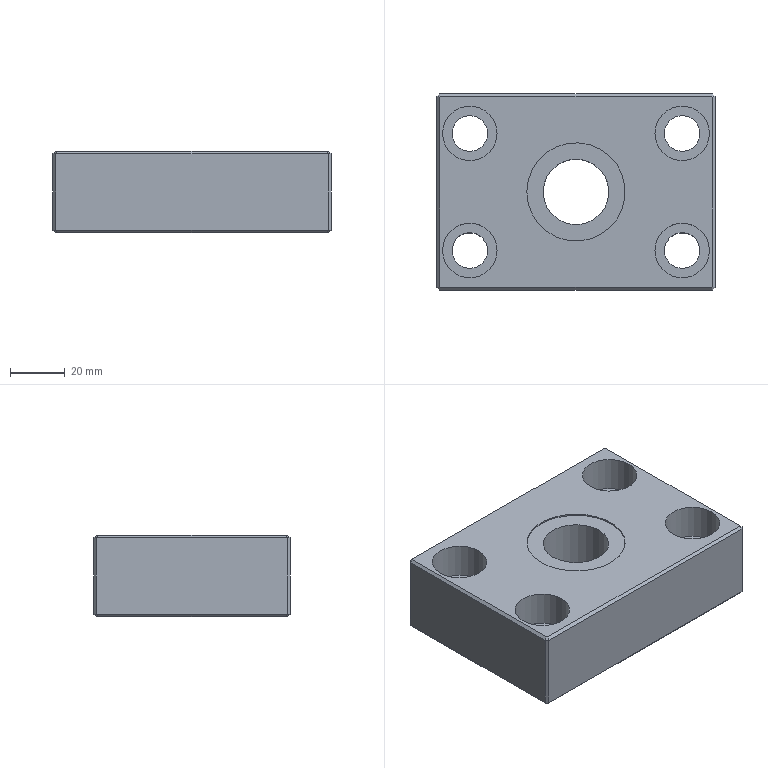NC program | NX | posted with a generic post | part box 102 x 72 x 30 mm
Whole program:
N10 G17 G21 G94 G90
(PLANAR_MILL , TOOL : D80-FACE-MILL)
N12 T01 M6
N14 G53
N16 G17 G0 G90 X96. Y-0.5 S3500 M3
N18 G43 Z20. H1
N20 Z2.03
N22 G94 G1 Z0.03 F800.
N24 X53.
N26 X-53.
N28 X-96.
N30 Z2.03
N32 G0 Z20.
N34 M5
(ADAPTIVE_MILLING , TOOL : D12-36-D12-75-3T-ROUGH)
N36 T02 M6
N38 G53
N40 G17 G0 G90 X-65.022 Y-0.963 S4500 M3
N42 G43 Z20. H2
N44 Z-28.
N46 G94 G1 X-64.873 Y-0.957 Z-28.937 F3000.
N48 X-64.723 Y-0.951 Z-29.308
N50 X-64.573 Y-0.945 Z-29.58
N52 X-64.423 Y-0.939 Z-29.8
N54 X-64.273 Y-0.932 Z-29.984
N56 X-64.123 Y-0.926 Z-30.142
N58 X-63.973 Y-0.92 Z-30.28
N60 X-63.823 Y-0.914 Z-30.4
N62 X-63.673 Y-0.908 Z-30.505
N64 X-63.524 Y-0.902 Z-30.598
N66 X-63.374 Y-0.896 Z-30.679
N68 X-63.224 Y-0.89 Z-30.75
N70 X-63.074 Y-0.884 Z-30.81
N72 X-62.924 Y-0.878 Z-30.862
N74 X-62.774 Y-0.872 Z-30.905
N76 X-62.624 Y-0.866 Z-30.939
N78 X-62.474 Y-0.86 Z-30.966
N80 X-62.325 Y-0.854 Z-30.985
N82 X-62.175 Y-0.848 Z-30.996
N84 X-62.025 Y-0.842 Z-31.
N86 X-60.086 Y-0.763
N88 G3 X-59.024 Y-0.037 R1.213
N90 X-58.336 Y3.017 R10.296
N92 X-58.027 Y11.039 R88.278
N94 G1 X-58.001 Y22.999
N96 G2 X-57.983 Y34.698 R876.175
N98 X-55.786 Y38.926 R6.62
N100 G3 X-54.348 Y40.349 R38.231
N102 G1 X-53.415 Y41.114
N104 X-52.352 Y41.682
N106 X-51.198 Y42.032
N108 G2 X-41.908 Y42.469 R88.797
N110 G1 X-28.858 Y42.499
N112 X49.797
N114 G2 X54.262 Y40.49 R6.403
N116 G3 X55.349 Y39.348 R52.182
N118 G1 X56.114 Y38.415
N120 X56.682 Y37.352
N122 G2 X57.709 Y31.906 R22.458
N124 X57.984 Y22.313 R130.619
N126 G1 X57.999 Y11.513
N128 X57.998 Y-34.397
N130 G2 X56.106 Y-38.609 R6.375
N132 G3 X54.348 Y-40.349 R75.716
N134 G1 X53.415 Y-41.114
N136 X52.352 Y-41.682
N138 X51.198 Y-42.032
N140 G2 X42.058 Y-42.467 R87.641
N142 G1 X28.858 Y-42.499
N144 X-49.901 Y-42.498
N146 G2 X-54.172 Y-40.545 R6.4
N148 G1 X-55.349 Y-39.348
N150 X-56.114 Y-38.415
N152 X-56.682 Y-37.352
N154 G2 X-57.712 Y-31.831 R22.603
N156 X-57.981 Y-22.837 R125.592
N158 G1 X-57.999 Y-11.437
N160 X-57.994 Y30.263
N162 G2 X-57.654 Y31.418 R35.846
N164 X-57.159 Y33.447 R34.168
N166 X-57.031 Y36.201 R19.38
N168 G1 X-56.681 Y37.355
N170 X-56.113 Y38.418
N172 X-55.399 Y39.287
N174 X-56.113 Y38.418
N176 X-56.681 Y37.355
N178 X-57.031 Y36.201
N180 G3 X-57.15 Y33.525 R16.38
N182 G2 X-57.284 Y30.611 R46.933
N184 G3 X-57.399 Y18.162 R360.152
N186 G1 Y-30.651
N188 X-57.15 Y-32.257
N190 Y-35.
N192 X-57.032 Y-36.198
N194 X-57.15 Y-35.
N196 Y35.001
N198 X-57.031 Y36.201
N200 X-56.681 Y37.355
N202 X-56.113 Y38.418
N204 G2 X-53.415 Y41.114 R14.478
N206 G1 X-52.352 Y41.682
N208 X-51.198 Y42.032
N210 X-49.999 Y42.15
N212 X50.001
N214 X51.201 Y42.031
N216 X52.355 Y41.681
N218 X53.418 Y41.113
N220 G2 X56.114 Y38.415 R14.476
N222 G1 X56.682 Y37.352
N224 X57.032 Y36.198
N226 X57.15 Y34.999
N228 Y-35.001
N230 X57.031 Y-36.201
N232 X56.681 Y-37.355
N234 X56.113 Y-38.418
N236 G2 X53.415 Y-41.114 R14.478
N238 G1 X52.352 Y-41.682
N240 X51.198 Y-42.032
N242 X49.999 Y-42.15
N244 X-50.001
N246 X-51.201 Y-42.031
N248 X-52.355 Y-41.681
N250 X-53.418 Y-41.113
N252 G2 X-54.614 Y-40.083 R11.256
N254 G3 X-56.113 Y-39.912 R1.212
N256 G1 X-57.83 Y-40.984
N258 X-57.958 Y-41.063 Z-30.996
N260 X-58.085 Y-41.143 Z-30.985
N262 X-58.212 Y-41.222 Z-30.966
N264 X-58.339 Y-41.302 Z-30.939
N266 X-58.466 Y-41.381 Z-30.905
N268 X-58.594 Y-41.461 Z-30.862
N270 X-58.721 Y-41.54 Z-30.81
N272 X-58.848 Y-41.62 Z-30.75
N274 X-58.975 Y-41.699 Z-30.679
N276 X-59.103 Y-41.779 Z-30.598
N278 X-59.23 Y-41.858 Z-30.505
N280 X-59.357 Y-41.937 Z-30.4
N282 X-59.484 Y-42.017 Z-30.28
N284 X-59.612 Y-42.096 Z-30.142
N286 X-59.739 Y-42.176 Z-29.984
N288 X-59.866 Y-42.255 Z-29.8
N290 X-59.993 Y-42.335 Z-29.58
N292 X-60.12 Y-42.414 Z-29.308
N294 X-60.248 Y-42.494 Z-28.937
N296 X-60.375 Y-42.573 Z-28.
N298 G0 Z20.
N300 X-4.55 Y-2.906
N302 Z3.
N304 G3 X-4.55 Y-2.906 Z2.408 I4.55 J2.908
N306 X-4.55 Y-2.906 Z1.816 I4.55 J2.908
N308 X-4.55 Y-2.906 Z1.223 I4.55 J2.908
N310 X-4.55 Y-2.906 Z0.631 I4.55 J2.908
N312 X-4.55 Y-2.906 Z0.039 I4.55 J2.908
N314 X-4.55 Y-2.906 Z-0.553 I4.55 J2.908
N316 X-4.55 Y-2.906 Z-1.146 I4.55 J2.908
N318 X-4.55 Y-2.906 Z-1.738 I4.55 J2.908
N320 X-4.55 Y-2.906 Z-2.33 I4.55 J2.908
N322 X-4.55 Y-2.906 Z-2.922 I4.55 J2.908
N324 X-4.55 Y-2.906 Z-3.515 I4.55 J2.908
N326 X-4.55 Y-2.906 Z-4.107 I4.55 J2.908
N328 X-4.55 Y-2.906 Z-4.699 I4.55 J2.908
N330 X-4.55 Y-2.906 Z-5.291 I4.55 J2.908
N332 X-4.55 Y-2.906 Z-5.884 I4.55 J2.908
N334 X-4.55 Y-2.906 Z-6.476 I4.55 J2.908
N336 X-4.55 Y-2.906 Z-7.068 I4.55 J2.908
N338 X-4.55 Y-2.906 Z-7.66 I4.55 J2.908
N340 X-4.55 Y-2.906 Z-8.252 I4.55 J2.908
N342 X-4.55 Y-2.906 Z-8.845 I4.55 J2.908
N344 X-4.55 Y-2.906 Z-9.437 I4.55 J2.908
N346 X-4.55 Y-2.906 Z-10.029 I4.55 J2.908
N348 X-4.55 Y-2.906 Z-10.621 I4.55 J2.908
N350 X-4.55 Y-2.906 Z-11.214 I4.55 J2.908
N352 X-4.55 Y-2.906 Z-11.806 I4.55 J2.908
N354 X-4.55 Y-2.906 Z-12.398 I4.55 J2.908
N356 X-4.55 Y-2.906 Z-12.99 I4.55 J2.908
N358 X-4.55 Y-2.906 Z-13.583 I4.55 J2.908
N360 X-4.55 Y-2.906 Z-14.175 I4.55 J2.908
N362 X-4.55 Y-2.906 Z-14.767 I4.55 J2.908
N364 X-4.55 Y-2.906 Z-15.359 I4.55 J2.908
N366 X-4.55 Y-2.906 Z-15.952 I4.55 J2.908
N368 X-4.55 Y-2.906 Z-16.544 I4.55 J2.908
N370 X-4.55 Y-2.906 Z-17.136 I4.55 J2.908
N372 X-4.55 Y-2.906 Z-17.728 I4.55 J2.908
N374 X-4.55 Y-2.906 Z-18.321 I4.55 J2.908
N376 X-4.55 Y-2.906 Z-18.913 I4.55 J2.908
N378 X-4.55 Y-2.906 Z-19.505 I4.55 J2.908
N380 X-4.55 Y-2.906 Z-20.097 I4.55 J2.908
N382 X-4.55 Y-2.906 Z-20.689 I4.55 J2.908
N384 X-4.55 Y-2.906 Z-21.282 I4.55 J2.908
N386 X-4.55 Y-2.906 Z-21.874 I4.55 J2.908
N388 X-4.55 Y-2.906 Z-22.466 I4.55 J2.908
N390 X-4.55 Y-2.906 Z-23.058 I4.55 J2.908
N392 X-4.55 Y-2.906 Z-23.651 I4.55 J2.908
N394 X-4.55 Y-2.906 Z-24.243 I4.55 J2.908
N396 X-4.55 Y-2.906 Z-24.835 I4.55 J2.908
N398 X-4.55 Y-2.906 Z-25.427 I4.55 J2.908
N400 X-4.55 Y-2.906 Z-26.02 I4.55 J2.908
N402 X-4.55 Y-2.906 Z-26.612 I4.55 J2.908
N404 X-4.55 Y-2.906 Z-27.204 I4.55 J2.908
N406 X-4.55 Y-2.906 Z-27.796 I4.55 J2.908
N408 X-4.55 Y-2.906 Z-28.389 I4.55 J2.908
N410 X-4.55 Y-2.906 Z-28.981 I4.55 J2.908
N412 X-4.55 Y-2.906 Z-29.573 I4.55 J2.908
N414 X-4.55 Y-2.906 Z-30.165 I4.55 J2.908
N416 X-4.55 Y-2.906 Z-30.757 I4.55 J2.908
N418 X5.4 Y0.001 Z-31. R5.4
N420 X-1.556 Y-5.216 R-5.422
N422 X4.807 Y-2.623 R5.524
N424 X4.62 Y3.544 R5.618
N426 X-3.378 Y4.764 R5.831
N428 X-3.409 Y-4.741 R5.854
N430 X4.723 Y-3.435 R5.871
N432 X4.435 Y3.792 R5.865
N434 X2.579 Y3.657 R1.212
N436 G1 X1.641 Y2.352
N438 X1.554 Y2.23 Z-30.996
N440 X1.466 Y2.108 Z-30.985
N442 X1.378 Y1.987 Z-30.966
N444 X1.291 Y1.865 Z-30.939
N446 X1.203 Y1.743 Z-30.905
N448 X1.116 Y1.621 Z-30.862
N450 X1.028 Y1.499 Z-30.81
N452 X0.941 Y1.378 Z-30.75
N454 X0.853 Y1.256 Z-30.679
N456 X0.765 Y1.134 Z-30.598
N458 X0.678 Y1.012 Z-30.505
N460 X0.59 Y0.891 Z-30.4
N462 X0.503 Y0.769 Z-30.28
N464 X0.415 Y0.647 Z-30.142
N466 X0.328 Y0.525 Z-29.984
N468 X0.24 Y0.403 Z-29.8
N470 X0.152 Y0.282 Z-29.58
N472 X0.065 Y0.16 Z-29.308
N474 X-0.023 Y0.038 Z-28.937
N476 X-0.11 Y-0.084 Z-28.
N478 G0 Z20.
(PLANAR_MILL_2 , TOOL : D12-36-D12-75-3T-ROUGH)
N480 X10.73 Y-5.177
N482 Z1.
N484 G1 X10.829 Y-5.006 Z0.997 F1000.
N486 X11.553 Y-2.975 Z0.959
N488 X11.9 Y-0.846 Z0.921
N490 Y0.846 Z0.892
N492 X11.553 Y2.975 Z0.854
N494 X10.829 Y5.006 Z0.816
N496 X9.75 Y6.875 Z0.779
N498 X8.353 Y8.518 Z0.741
N500 X6.682 Y9.883 Z0.703
N502 X5.218 Y10.728 Z0.674
N504 X3.037 Y11.537 Z0.633
N506 X0.741 Y11.907 Z0.593
N508 X-1.583 Y11.824 Z0.552
N510 X-3.847 Y11.293 Z0.512
N512 X-5.965 Y10.332 Z0.471
N514 X-7.856 Y8.978 Z0.43
N516 X-9.449 Y7.283 Z0.39
N518 X-10.682 Y5.312 Z0.349
N520 X-11.51 Y3.138 Z0.309
N522 X-11.9 Y0.846 Z0.268
N524 Y-0.846 Z0.238
N526 X-11.51 Y-3.138 Z0.198
N528 X-10.682 Y-5.312 Z0.157
N530 X-9.449 Y-7.283 Z0.117
N532 X-7.856 Y-8.978 Z0.076
N534 X-5.965 Y-10.332 Z0.036
N536 X-3.847 Y-11.293 Z-0.005
N538 X-1.583 Y-11.824 Z-0.046
N540 X0.741 Y-11.907 Z-0.086
N542 X3.037 Y-11.537 Z-0.127
N544 X5.218 Y-10.728 Z-0.167
N546 X6.682 Y-9.883 Z-0.197
N548 X8.353 Y-8.518 Z-0.235
N550 X9.75 Y-6.875 Z-0.272
N552 X10.829 Y-5.006 Z-0.31
N554 X11.553 Y-2.975 Z-0.348
N556 X11.9 Y-0.846 Z-0.385
N558 Y0. Z-0.4
N560 G3 X0. Y11.9 R11.9
N562 X11.9 Y0. R-11.9
N564 G1 Z0.6
N566 G0 Z20.
(PLANAR_MILL_2_COPY_COPY_COPY , TOOL : D12-36-D12-75-3T-ROUGH)
N568 X-3.75 Y2. S4000
N570 Z-18.5
N572 G1 Z-20.5 F800.
N574 X-4.25
N576 G3 X-6.25 Y0. R2.
N578 X0. Y-6.25 R6.25
N580 X-6.25 Y0. R-6.25
N582 X-4.25 Y-2. R2.
N584 G1 X-3.75
N586 Z-18.5
N588 G0 Z20.
N590 M5
(PLANAR_MILL_1 , TOOL : D12-36-D12-120-3T-FINISH)
N592 T03 M6
N594 G53
N596 G17 G0 G90 X55.292 Y-42. S4000 M3
N598 G43 Z20. H3
N600 Z-29.
N602 G94 G1 Z-31. F800.
N604 X49.999
N606 X-50.
N608 G2 X-54.243 Y-40.243 R6.
N610 G1 X-55.243 Y-39.243
N612 G2 X-57. Y-35. R6.
N614 G1 Y35.
N616 G2 X-55.243 Y39.243 R6.
N618 G1 X-54.243 Y40.243
N620 G2 X-50. Y42. R6.
N622 G1 X50.
N624 G2 X54.243 Y40.243 R6.
N626 G1 X55.243 Y39.243
N628 G2 X57. Y35. R6.
N630 G1 Y-35.
N632 G2 X55.243 Y-39.243 R6.
N634 G1 X54.244 Y-40.242
N636 X50.501 Y-43.984
N638 Z-29.
N640 G0 Z20.
N642 X55.292 Y-42.
N644 Z-29.
N646 G1 Z-31.
N648 X49.999
N650 X-50.
N652 G2 X-54.243 Y-40.243 R6.
N654 G1 X-55.243 Y-39.243
N656 G2 X-57. Y-35. R6.
N658 G1 Y35.
N660 G2 X-55.243 Y39.243 R6.
N662 G1 X-54.243 Y40.243
N664 G2 X-50. Y42. R6.
N666 G1 X50.
N668 G2 X54.243 Y40.243 R6.
N670 G1 X55.243 Y39.243
N672 G2 X57. Y35. R6.
N674 G1 Y-35.
N676 G2 X55.243 Y-39.243 R6.
N678 G1 X54.244 Y-40.242
N680 X50.501 Y-43.984
N682 Z-29.
N684 G0 Z20.
(PLANAR_MILL_2_COPY , TOOL : D12-36-D12-120-3T-FINISH)
N686 X4.583 Y-2. S4400
N688 Z1.5
N690 G1 Z-0.5 F300.
N692 X10.
N694 G3 X12. Y0. R2.
N696 X0. Y12. R12.
N698 X12. Y0. R-12.
N700 X10. Y2. R2.
N702 G1 X4.583
N704 Z1.5
N706 G0 Z20.
(PLANAR_MILL_2_COPY_COPY , TOOL : D12-36-D12-120-3T-FINISH)
N708 X-3.464 S4000
N710 Z-28.5
N712 G1 Z-30.5 F800.
N714 X-4.
N716 G3 X-6. Y0. R2.
N718 X0. Y-6. R6.
N720 X-6. Y0. R-6.
N722 X-4. Y-2. R2.
N724 G1 X-3.464
N726 Z-28.5
N728 G0 Z20.
N730 M5
(DRILLING , TOOL : CHAMFER-D10-90DEG)
N732 T04 M6
N734 G53
N736 G17 G0 G90 X-38.9 Y21.45 S2000 M3
N738 G43 Z20. H4
N740 G94 G81 G99 Z-1.5 F200. R3.
N742 Y-21.45
N744 X38.9
N746 Y21.45
N748 G80
N750 G0 X38.9 Y21.45 Z20.
N752 M5
(DRILLING_COPY , TOOL : D13DRILL )
N754 T06 M6
N756 G53
N758 G17 G0 G90 X-38.9 Y21.45 S1600 M3
N760 G43 Z20. H6
N762 G94 G83 G99 Z-35. F200. Q5. R3.
N764 Y-21.45
N766 X38.9
N768 Y21.45
N770 G80
N772 G0 X38.9 Y21.45 Z20.
N774 M5
(DRILLING_COPY_COPY , TOOL : D20PLUNGE-MILL)
N776 T07 M6
N778 G53
N780 G17 G0 G90 X-38.9 Y21.45 S1200 M3
N782 G43 Z20. H7
N784 G94 G81 G99 Z-13. F60. R3.
N786 Y-21.45
N788 X38.9
N790 Y21.45
N792 G80
N794 G0 X38.9 Y21.45 Z20.
N796 M5
(PLANAR_MILL_3 , TOOL : CHAMFER-D6-90DEG)
N798 T05 M6
N800 G53
N802 G17 G0 G90 X-32.715 Y19.45 S3000 M3
N804 G43 Z20. H5
N806 Z0.5
N808 G94 G1 Z-1.5 F1000.
N810 X-32.4
N812 G3 X-30.4 Y21.45 R2.
N814 X-38.9 Y29.95 R8.5
N816 X-30.4 Y21.45 R-8.5
N818 X-32.4 Y23.45 R2.
N820 G1 X-32.715
N822 Z0.5
N824 G0 Z20.
N826 Y-23.45
N828 Z0.5
N830 G1 Z-1.5
N832 X-32.4
N834 G3 X-30.4 Y-21.45 R2.
N836 X-38.9 Y-12.95 R8.5
N838 X-30.4 Y-21.45 R-8.5
N840 X-32.4 Y-19.45 R2.
N842 G1 X-32.715
N844 Z0.5
N846 G0 Z20.
N848 X45.085 Y-23.45
N850 Z0.5
N852 G1 Z-1.5
N854 X45.4
N856 G3 X47.4 Y-21.45 R2.
N858 X38.9 Y-12.95 R8.5
N860 X47.4 Y-21.45 R-8.5
N862 X45.4 Y-19.45 R2.
N864 G1 X45.085
N866 Z0.5
N868 G0 Z20.
N870 Y19.45
N872 Z0.5
N874 G1 Z-1.5
N876 X45.4
N878 G3 X47.4 Y21.45 R2.
N880 X38.9 Y29.95 R8.5
N882 X47.4 Y21.45 R-8.5
N884 X45.4 Y23.45 R2.
N886 G1 X45.085
N888 Z0.5
N890 G0 Z20.
(PLANAR_MILL_3_COPY_1 , TOOL : CHAMFER-D6-90DEG)
N892 X36.531 Y-19.45
N894 Z-12.5
N896 G1 Z-14.5
N898 X35.8
N900 G3 X33.8 Y-21.45 R2.
N902 X38.9 Y-26.55 R5.1
N904 X33.8 Y-21.45 R-5.1
N906 X35.8 Y-23.45 R2.
N908 G1 X36.531
N910 Z-12.5
N912 G0 Z20.
N914 Y23.45
N916 Z-12.5
N918 G1 Z-14.5
N920 X35.8
N922 G3 X33.8 Y21.45 R2.
N924 X38.9 Y16.35 R5.1
N926 X33.8 Y21.45 R-5.1
N928 X35.8 Y19.45 R2.
N930 G1 X36.531
N932 Z-12.5
N934 G0 Z20.
N936 X-41.269 Y23.45
N938 Z-12.5
N940 G1 Z-14.5
N942 X-42.
N944 G3 X-44. Y21.45 R2.
N946 X-38.9 Y16.35 R5.1
N948 X-44. Y21.45 R-5.1
N950 X-42. Y19.45 R2.
N952 G1 X-41.269
N954 Z-12.5
N956 G0 Z20.
N958 Y-19.45
N960 Z-12.5
N962 G1 Z-14.5
N964 X-42.
N966 G3 X-44. Y-21.45 R2.
N968 X-38.9 Y-26.55 R5.1
N970 X-44. Y-21.45 R-5.1
N972 X-42. Y-23.45 R2.
N974 G1 X-41.269
N976 Z-12.5
N978 G0 Z20.
(PLANAR_MILL_3_COPY , TOOL : CHAMFER-D6-90DEG)
N980 X15.37 Y-2.
N982 Z1.6
N984 G1 Z-0.4
N986 X15.5
N988 G3 X17.5 Y0. R2.
N990 X0. Y17.5 R17.5
N992 X17.5 Y0. R-17.5
N994 X15.5 Y2. R2.
N996 G1 X15.37
N998 Z1.6
N1000 G0 Z20.
(PLANAR_MILL_3_COPY_COPY , TOOL : CHAMFER-D6-90DEG)
N1002 X-8.775
N1004 Z-0.8
N1006 G1 Z-2.8 F600.
N1008 X-9.
N1010 G3 X-11. Y0. R2.
N1012 X0. Y-11. R11.
N1014 X-11. Y0. R-11.
N1016 X-9. Y-2. R2.
N1018 G1 X-8.775
N1020 Z-0.8
N1022 G0 Z20.
(PLANAR_MILL_4 , TOOL : CHAMFER-D6-90DEG)
N1024 X53.828 Y-36.414
N1026 Z0.
N1028 G1 Z-2. F1000.
N1030 G3 X51. Y-36.414 R2.
N1032 G2 X49.586 Y-37. R2.
N1034 G1 X-49.586
N1036 G2 X-51. Y-36.414 R2.
N1038 G1 X-51.414 Y-36.
N1040 G2 X-52. Y-34.586 R2.
N1042 G1 Y34.586
N1044 G2 X-51.414 Y36. R2.
N1046 G1 X-51. Y36.414
N1048 G2 X-49.586 Y37. R2.
N1050 G1 X49.586
N1052 G2 X51. Y36.414 R2.
N1054 G1 X51.414 Y36.
N1056 G2 X52. Y34.586 R2.
N1058 G1 Y-34.586
N1060 G2 X51.414 Y-36. R2.
N1062 G1 X51. Y-36.414
N1064 G3 X51. Y-39.243 R2.
N1066 G1 Z0.
N1068 G0 Z20.
N1070 M5
(THREAD_MILLING , TOOL : G3-4)
N1072 T08 M6
N1074 G53
N1076 G17 G0 G90 X0. Y0. S4000 M3
N1078 G43 Z20. H8
N1080 Z-18.078
N1082 G41 G94 G1 X3.745 Y1.089 F300. D8
N1084 G3 X4.092 Y2.156 Z-18. R0.783
N1086 X4.092 Y2.156 Z-16.186 I-4.092 J-2.156
N1088 X3.015 Y2.473 Z-16.108 R0.783
N1090 G40
N1092 G1 X0. Y0.
N1094 G0 Z-18.098
N1096 G41 G1 X3.799 Y0.88
N1098 G3 X4.291 Y2.261 Z-18. R0.996
N1100 X4.291 Y2.261 Z-16.186 I-4.291 J-2.261
N1102 X2.874 Y2.636 Z-16.088 R0.996
N1104 G40
N1106 G1 X0. Y0.
N1108 G0 Z-18.116
N1110 G41 G1 X3.84 Y0.68
N1112 G3 X4.49 Y2.366 Z-18. R1.199
N1114 X4.49 Y2.366 Z-16.186 I-4.49 J-2.366
N1116 X2.733 Y2.783 Z-16.07 R1.199
N1118 G40
N1120 G1 X0. Y0.
N1122 G0 Z-18.133
N1124 G41 G1 X3.869 Y0.491
N1126 G3 X4.689 Y2.471 Z-18. R1.393
N1128 X4.689 Y2.471 Z-16.186 I-4.689 J-2.471
N1130 X2.592 Y2.914 Z-16.053 R1.393
N1132 G40
N1134 G1 X0. Y0.
N1136 G0 Z-18.133
N1138 G41 G1 X3.869 Y0.491
N1140 G3 X4.689 Y2.471 Z-18. R1.393
N1142 X4.689 Y2.471 Z-16.186 I-4.689 J-2.471
N1144 X2.592 Y2.914 Z-16.053 R1.393
N1146 G40
N1148 G1 X0. Y0.
N1150 G0 Z-18.133
N1152 G41 G1 X3.869 Y0.491
N1154 G3 X4.689 Y2.471 Z-18. R1.393
N1156 X4.689 Y2.471 Z-16.186 I-4.689 J-2.471
N1158 X2.592 Y2.914 Z-16.053 R1.393
N1160 G40
N1162 G1 X0. Y0.
N1164 G0 Z20.
N1166 M5
(PLANAR_MILL_COPY , TOOL : D80-FACE-MILL)
N1168 T01 M6
N1170 G53
N1172 G17 G0 G90 X96. Y-0.5 S4500 M3
N1174 G43 Z20. H1
N1176 Z2.
N1178 G94 G1 Z0. F600.
N1180 X53.
N1182 X-53.
N1184 X-96.
N1186 Z2.
N1188 G0 Z20.
N1190 M5
N1192 M2